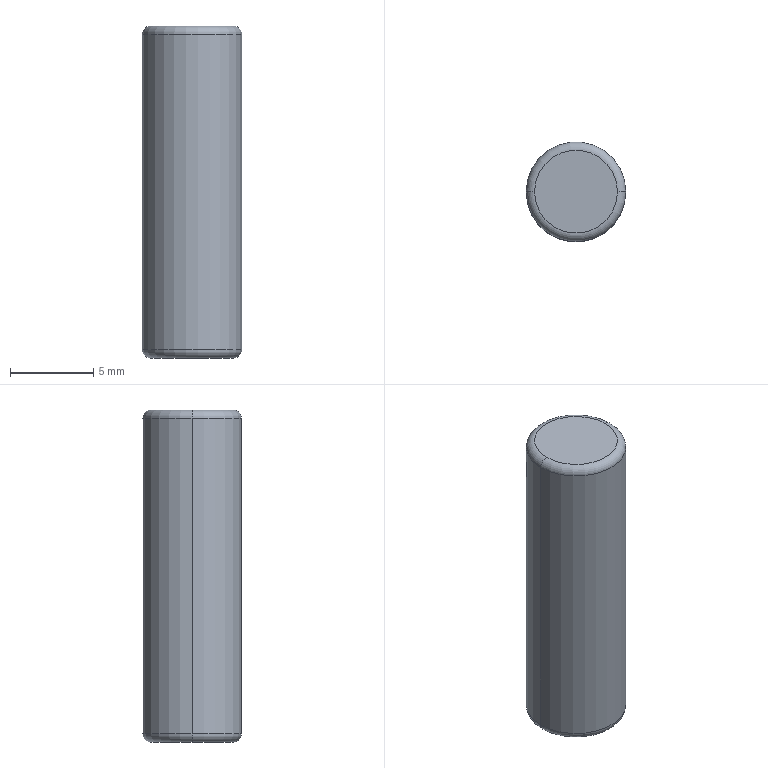Part | STEP file | 1 solid | 8 faces | box 6 x 6 x 20 mm | volume 563.539 mm3 | torus 4 | cylinder 2 | plane 2 | commonest cylinder face diameters 6 x2
STEP:
#1=CARTESIAN_POINT('',(0.,0.,0.));
#2=DIRECTION('',(0.,0.,1.));
#3=DIRECTION('',(1.,0.,0.));
#4=AXIS2_PLACEMENT_3D('',#1,#2,#3);
#5=CARTESIAN_POINT('',(-3.,0.,19.5));
#6=VERTEX_POINT('',#5);
#7=CARTESIAN_POINT('',(3.,0.,19.5));
#8=VERTEX_POINT('',#7);
#9=CARTESIAN_POINT('',(0.,0.,19.5));
#10=DIRECTION('',(0.,0.,-1.));
#11=DIRECTION('',(1.,0.,0.));
#12=AXIS2_PLACEMENT_3D('',#9,#10,#11);
#13=CIRCLE('',#12,3.);
#14=CARTESIAN_POINT('',(0.,0.,19.5));
#15=DIRECTION('',(0.,0.,1.));
#16=DIRECTION('',(1.,0.,0.));
#17=AXIS2_PLACEMENT_3D('',#14,#15,#16);
#18=TOROIDAL_SURFACE('',#17,2.5,0.5);
#19=CARTESIAN_POINT('',(6.283,0.));
#20=DIRECTION('',(-1.,0.));
#21=VECTOR('',#20,1.);
#22=LINE('',#19,#21);
#23=(GEOMETRIC_REPRESENTATION_CONTEXT(2)PARAMETRIC_REPRESENTATION_CONTEXT()REPRESENTATION_CONTEXT('',''));
#24=DEFINITIONAL_REPRESENTATION('',(#22),#23);
#25=PCURVE('',#18,#24);
#26=CARTESIAN_POINT('',(0.,0.,20.));
#27=DIRECTION('',(0.,0.,-1.));
#28=DIRECTION('',(-1.,0.,0.));
#29=AXIS2_PLACEMENT_3D('',#26,#27,#28);
#30=CYLINDRICAL_SURFACE('',#29,3.);
#31=CARTESIAN_POINT('',(-3.142,0.5));
#32=DIRECTION('',(1.,0.));
#33=VECTOR('',#32,1.);
#34=LINE('',#31,#33);
#35=(GEOMETRIC_REPRESENTATION_CONTEXT(2)PARAMETRIC_REPRESENTATION_CONTEXT()REPRESENTATION_CONTEXT('',''));
#36=DEFINITIONAL_REPRESENTATION('',(#34),#35);
#37=PCURVE('',#30,#36);
#38=SURFACE_CURVE('',#13,(#25,#37),.PCURVE_S1.);
#39=EDGE_CURVE('',#6,#8,#38,.T.);
#40=ORIENTED_EDGE('',*,*,#39,.F.);
#41=CARTESIAN_POINT('',(-2.5,0.,20.));
#42=VERTEX_POINT('',#41);
#43=CARTESIAN_POINT('',(-2.5,0.,19.5));
#44=DIRECTION('',(0.,1.,0.));
#45=DIRECTION('',(-1.,0.,0.));
#46=AXIS2_PLACEMENT_3D('',#43,#44,#45);
#47=CIRCLE('',#46,0.5);
#48=CARTESIAN_POINT('',(3.142,0.));
#49=DIRECTION('',(0.,1.));
#50=VECTOR('',#49,1.);
#51=LINE('',#48,#50);
#52=(GEOMETRIC_REPRESENTATION_CONTEXT(2)PARAMETRIC_REPRESENTATION_CONTEXT()REPRESENTATION_CONTEXT('',''));
#53=DEFINITIONAL_REPRESENTATION('',(#51),#52);
#54=PCURVE('',#18,#53);
#55=CARTESIAN_POINT('',(0.,0.,19.5));
#56=DIRECTION('',(0.,0.,1.));
#57=DIRECTION('',(1.,0.,0.));
#58=AXIS2_PLACEMENT_3D('',#55,#56,#57);
#59=TOROIDAL_SURFACE('',#58,2.5,0.5);
#60=CARTESIAN_POINT('',(3.142,0.));
#61=DIRECTION('',(0.,1.));
#62=VECTOR('',#61,1.);
#63=LINE('',#60,#62);
#64=(GEOMETRIC_REPRESENTATION_CONTEXT(2)PARAMETRIC_REPRESENTATION_CONTEXT()REPRESENTATION_CONTEXT('',''));
#65=DEFINITIONAL_REPRESENTATION('',(#63),#64);
#66=PCURVE('',#59,#65);
#67=SURFACE_CURVE('',#47,(#54,#66),.PCURVE_S1.);
#68=EDGE_CURVE('',#6,#42,#67,.T.);
#69=ORIENTED_EDGE('',*,*,#68,.T.);
#70=CARTESIAN_POINT('',(2.5,0.,20.));
#71=VERTEX_POINT('',#70);
#72=CARTESIAN_POINT('',(0.,0.,20.));
#73=DIRECTION('',(0.,0.,1.));
#74=DIRECTION('',(1.,0.,0.));
#75=AXIS2_PLACEMENT_3D('',#72,#73,#74);
#76=CIRCLE('',#75,2.5);
#77=CARTESIAN_POINT('',(0.,1.571));
#78=DIRECTION('',(1.,0.));
#79=VECTOR('',#78,1.);
#80=LINE('',#77,#79);
#81=(GEOMETRIC_REPRESENTATION_CONTEXT(2)PARAMETRIC_REPRESENTATION_CONTEXT()REPRESENTATION_CONTEXT('',''));
#82=DEFINITIONAL_REPRESENTATION('',(#80),#81);
#83=PCURVE('',#18,#82);
#84=CARTESIAN_POINT('',(0.,0.,20.));
#85=DIRECTION('',(0.,0.,1.));
#86=DIRECTION('',(1.,0.,0.));
#87=AXIS2_PLACEMENT_3D('',#84,#85,#86);
#88=PLANE('',#87);
#89=CARTESIAN_POINT('',(0.,0.));
#90=DIRECTION('',(1.,0.));
#91=AXIS2_PLACEMENT_2D('',#89,#90);
#92=CIRCLE('',#91,2.5);
#93=(GEOMETRIC_REPRESENTATION_CONTEXT(2)PARAMETRIC_REPRESENTATION_CONTEXT()REPRESENTATION_CONTEXT('',''));
#94=DEFINITIONAL_REPRESENTATION('',(#92),#93);
#95=PCURVE('',#88,#94);
#96=SURFACE_CURVE('',#76,(#83,#95),.PCURVE_S1.);
#97=EDGE_CURVE('',#71,#42,#96,.T.);
#98=ORIENTED_EDGE('',*,*,#97,.F.);
#99=CARTESIAN_POINT('',(2.5,0.,19.5));
#100=DIRECTION('',(0.,-1.,0.));
#101=DIRECTION('',(0.,0.,-1.));
#102=AXIS2_PLACEMENT_3D('',#99,#100,#101);
#103=CIRCLE('',#102,0.5);
#104=CARTESIAN_POINT('',(0.,-1.571));
#105=DIRECTION('',(0.,1.));
#106=VECTOR('',#105,1.);
#107=LINE('',#104,#106);
#108=(GEOMETRIC_REPRESENTATION_CONTEXT(2)PARAMETRIC_REPRESENTATION_CONTEXT()REPRESENTATION_CONTEXT('',''));
#109=DEFINITIONAL_REPRESENTATION('',(#107),#108);
#110=PCURVE('',#18,#109);
#111=CARTESIAN_POINT('',(6.283,-1.571));
#112=DIRECTION('',(0.,1.));
#113=VECTOR('',#112,1.);
#114=LINE('',#111,#113);
#115=(GEOMETRIC_REPRESENTATION_CONTEXT(2)PARAMETRIC_REPRESENTATION_CONTEXT()REPRESENTATION_CONTEXT('',''));
#116=DEFINITIONAL_REPRESENTATION('',(#114),#115);
#117=PCURVE('',#59,#116);
#118=SURFACE_CURVE('',#103,(#110,#117),.PCURVE_S1.);
#119=EDGE_CURVE('',#8,#71,#118,.T.);
#120=ORIENTED_EDGE('',*,*,#119,.F.);
#121=EDGE_LOOP('',(#40,#69,#98,#120));
#122=FACE_BOUND('',#121,.T.);
#123=ADVANCED_FACE('',(#122),#18,.T.);
#124=CARTESIAN_POINT('',(-2.5,0.,0.));
#125=VERTEX_POINT('',#124);
#126=CARTESIAN_POINT('',(2.5,0.,0.));
#127=VERTEX_POINT('',#126);
#128=CARTESIAN_POINT('',(0.,0.,0.));
#129=DIRECTION('',(0.,0.,-1.));
#130=DIRECTION('',(1.,0.,0.));
#131=AXIS2_PLACEMENT_3D('',#128,#129,#130);
#132=CIRCLE('',#131,2.5);
#133=CARTESIAN_POINT('',(0.,0.,0.5));
#134=DIRECTION('',(0.,0.,1.));
#135=DIRECTION('',(1.,0.,0.));
#136=AXIS2_PLACEMENT_3D('',#133,#134,#135);
#137=TOROIDAL_SURFACE('',#136,2.5,0.5);
#138=CARTESIAN_POINT('',(6.283,4.712));
#139=DIRECTION('',(-1.,0.));
#140=VECTOR('',#139,1.);
#141=LINE('',#138,#140);
#142=(GEOMETRIC_REPRESENTATION_CONTEXT(2)PARAMETRIC_REPRESENTATION_CONTEXT()REPRESENTATION_CONTEXT('',''));
#143=DEFINITIONAL_REPRESENTATION('',(#141),#142);
#144=PCURVE('',#137,#143);
#145=CARTESIAN_POINT('',(0.,0.,0.));
#146=DIRECTION('',(0.,0.,1.));
#147=DIRECTION('',(1.,0.,0.));
#148=AXIS2_PLACEMENT_3D('',#145,#146,#147);
#149=PLANE('',#148);
#150=CARTESIAN_POINT('',(2.5,0.));
#151=CARTESIAN_POINT('',(2.5,-4.33));
#152=CARTESIAN_POINT('',(-1.25,-2.165));
#153=CARTESIAN_POINT('',(-5.,0.));
#154=CARTESIAN_POINT('',(-1.25,2.165));
#155=CARTESIAN_POINT('',(2.5,4.33));
#156=CARTESIAN_POINT('',(2.5,0.));
#157=(BOUNDED_CURVE()B_SPLINE_CURVE(2,(#150,#151,#152,#153,#154,#155,#156),.UNSPECIFIED.,.T.,.F.)B_SPLINE_CURVE_WITH_KNOTS((1,2,2,2,2,1),(-2.094,0.,2.094,4.189,6.283,8.378),.UNSPECIFIED.)CURVE()GEOMETRIC_REPRESENTATION_ITEM()RATIONAL_B_SPLINE_CURVE((1.,0.5,1.,0.5,1.,0.5,1.))REPRESENTATION_ITEM(''));
#158=(GEOMETRIC_REPRESENTATION_CONTEXT(2)PARAMETRIC_REPRESENTATION_CONTEXT()REPRESENTATION_CONTEXT('',''));
#159=DEFINITIONAL_REPRESENTATION('',(#157),#158);
#160=PCURVE('',#149,#159);
#161=SURFACE_CURVE('',#132,(#144,#160),.PCURVE_S1.);
#162=EDGE_CURVE('',#125,#127,#161,.T.);
#163=ORIENTED_EDGE('',*,*,#162,.F.);
#164=CARTESIAN_POINT('',(-3.,0.,0.5));
#165=VERTEX_POINT('',#164);
#166=CARTESIAN_POINT('',(-2.5,0.,0.5));
#167=DIRECTION('',(0.,1.,0.));
#168=DIRECTION('',(-1.,0.,0.));
#169=AXIS2_PLACEMENT_3D('',#166,#167,#168);
#170=CIRCLE('',#169,0.5);
#171=CARTESIAN_POINT('',(3.142,0.));
#172=DIRECTION('',(0.,1.));
#173=VECTOR('',#172,1.);
#174=LINE('',#171,#173);
#175=(GEOMETRIC_REPRESENTATION_CONTEXT(2)PARAMETRIC_REPRESENTATION_CONTEXT()REPRESENTATION_CONTEXT('',''));
#176=DEFINITIONAL_REPRESENTATION('',(#174),#175);
#177=PCURVE('',#137,#176);
#178=CARTESIAN_POINT('',(0.,0.,0.5));
#179=DIRECTION('',(0.,0.,1.));
#180=DIRECTION('',(1.,0.,0.));
#181=AXIS2_PLACEMENT_3D('',#178,#179,#180);
#182=TOROIDAL_SURFACE('',#181,2.5,0.5);
#183=CARTESIAN_POINT('',(3.142,0.));
#184=DIRECTION('',(0.,1.));
#185=VECTOR('',#184,1.);
#186=LINE('',#183,#185);
#187=(GEOMETRIC_REPRESENTATION_CONTEXT(2)PARAMETRIC_REPRESENTATION_CONTEXT()REPRESENTATION_CONTEXT('',''));
#188=DEFINITIONAL_REPRESENTATION('',(#186),#187);
#189=PCURVE('',#182,#188);
#190=SURFACE_CURVE('',#170,(#177,#189),.PCURVE_S1.);
#191=EDGE_CURVE('',#125,#165,#190,.T.);
#192=ORIENTED_EDGE('',*,*,#191,.T.);
#193=CARTESIAN_POINT('',(3.,0.,0.5));
#194=VERTEX_POINT('',#193);
#195=CARTESIAN_POINT('',(0.,0.,0.5));
#196=DIRECTION('',(0.,0.,1.));
#197=DIRECTION('',(1.,0.,0.));
#198=AXIS2_PLACEMENT_3D('',#195,#196,#197);
#199=CIRCLE('',#198,3.);
#200=CARTESIAN_POINT('',(0.,6.283));
#201=DIRECTION('',(1.,0.));
#202=VECTOR('',#201,1.);
#203=LINE('',#200,#202);
#204=(GEOMETRIC_REPRESENTATION_CONTEXT(2)PARAMETRIC_REPRESENTATION_CONTEXT()REPRESENTATION_CONTEXT('',''));
#205=DEFINITIONAL_REPRESENTATION('',(#203),#204);
#206=PCURVE('',#137,#205);
#207=CARTESIAN_POINT('',(3.142,19.5));
#208=DIRECTION('',(-1.,0.));
#209=VECTOR('',#208,1.);
#210=LINE('',#207,#209);
#211=(GEOMETRIC_REPRESENTATION_CONTEXT(2)PARAMETRIC_REPRESENTATION_CONTEXT()REPRESENTATION_CONTEXT('',''));
#212=DEFINITIONAL_REPRESENTATION('',(#210),#211);
#213=PCURVE('',#30,#212);
#214=SURFACE_CURVE('',#199,(#206,#213),.PCURVE_S1.);
#215=EDGE_CURVE('',#194,#165,#214,.T.);
#216=ORIENTED_EDGE('',*,*,#215,.F.);
#217=CARTESIAN_POINT('',(2.5,0.,0.5));
#218=DIRECTION('',(0.,-1.,0.));
#219=DIRECTION('',(0.,0.,-1.));
#220=AXIS2_PLACEMENT_3D('',#217,#218,#219);
#221=CIRCLE('',#220,0.5);
#222=CARTESIAN_POINT('',(0.,4.712));
#223=DIRECTION('',(0.,1.));
#224=VECTOR('',#223,1.);
#225=LINE('',#222,#224);
#226=(GEOMETRIC_REPRESENTATION_CONTEXT(2)PARAMETRIC_REPRESENTATION_CONTEXT()REPRESENTATION_CONTEXT('',''));
#227=DEFINITIONAL_REPRESENTATION('',(#225),#226);
#228=PCURVE('',#137,#227);
#229=CARTESIAN_POINT('',(6.283,4.712));
#230=DIRECTION('',(0.,1.));
#231=VECTOR('',#230,1.);
#232=LINE('',#229,#231);
#233=(GEOMETRIC_REPRESENTATION_CONTEXT(2)PARAMETRIC_REPRESENTATION_CONTEXT()REPRESENTATION_CONTEXT('',''));
#234=DEFINITIONAL_REPRESENTATION('',(#232),#233);
#235=PCURVE('',#182,#234);
#236=SURFACE_CURVE('',#221,(#228,#235),.PCURVE_S1.);
#237=EDGE_CURVE('',#127,#194,#236,.T.);
#238=ORIENTED_EDGE('',*,*,#237,.F.);
#239=EDGE_LOOP('',(#163,#192,#216,#238));
#240=FACE_BOUND('',#239,.T.);
#241=ADVANCED_FACE('',(#240),#137,.T.);
#242=ORIENTED_EDGE('',*,*,#39,.T.);
#243=CARTESIAN_POINT('',(3.,0.,20.));
#244=DIRECTION('',(0.,0.,-1.));
#245=VECTOR('',#244,1.);
#246=LINE('',#243,#245);
#247=CARTESIAN_POINT('',(3.142,0.));
#248=DIRECTION('',(0.,1.));
#249=VECTOR('',#248,1.);
#250=LINE('',#247,#249);
#251=(GEOMETRIC_REPRESENTATION_CONTEXT(2)PARAMETRIC_REPRESENTATION_CONTEXT()REPRESENTATION_CONTEXT('',''));
#252=DEFINITIONAL_REPRESENTATION('',(#250),#251);
#253=PCURVE('',#30,#252);
#254=CARTESIAN_POINT('',(0.,0.,20.));
#255=DIRECTION('',(0.,0.,-1.));
#256=DIRECTION('',(-1.,0.,0.));
#257=AXIS2_PLACEMENT_3D('',#254,#255,#256);
#258=CYLINDRICAL_SURFACE('',#257,3.);
#259=CARTESIAN_POINT('',(3.142,0.));
#260=DIRECTION('',(0.,1.));
#261=VECTOR('',#260,1.);
#262=LINE('',#259,#261);
#263=(GEOMETRIC_REPRESENTATION_CONTEXT(2)PARAMETRIC_REPRESENTATION_CONTEXT()REPRESENTATION_CONTEXT('',''));
#264=DEFINITIONAL_REPRESENTATION('',(#262),#263);
#265=PCURVE('',#258,#264);
#266=SURFACE_CURVE('',#246,(#253,#265),.PCURVE_S1.);
#267=EDGE_CURVE('',#8,#194,#266,.T.);
#268=ORIENTED_EDGE('',*,*,#267,.T.);
#269=ORIENTED_EDGE('',*,*,#215,.T.);
#270=CARTESIAN_POINT('',(-3.,0.,20.));
#271=DIRECTION('',(0.,0.,-1.));
#272=VECTOR('',#271,1.);
#273=LINE('',#270,#272);
#274=CARTESIAN_POINT('',(0.,0.));
#275=DIRECTION('',(0.,1.));
#276=VECTOR('',#275,1.);
#277=LINE('',#274,#276);
#278=(GEOMETRIC_REPRESENTATION_CONTEXT(2)PARAMETRIC_REPRESENTATION_CONTEXT()REPRESENTATION_CONTEXT('',''));
#279=DEFINITIONAL_REPRESENTATION('',(#277),#278);
#280=PCURVE('',#30,#279);
#281=CARTESIAN_POINT('',(6.283,0.));
#282=DIRECTION('',(0.,1.));
#283=VECTOR('',#282,1.);
#284=LINE('',#281,#283);
#285=(GEOMETRIC_REPRESENTATION_CONTEXT(2)PARAMETRIC_REPRESENTATION_CONTEXT()REPRESENTATION_CONTEXT('',''));
#286=DEFINITIONAL_REPRESENTATION('',(#284),#285);
#287=PCURVE('',#258,#286);
#288=SURFACE_CURVE('',#273,(#280,#287),.PCURVE_S1.);
#289=EDGE_CURVE('',#6,#165,#288,.T.);
#290=ORIENTED_EDGE('',*,*,#289,.F.);
#291=EDGE_LOOP('',(#242,#268,#269,#290));
#292=FACE_BOUND('',#291,.T.);
#293=ADVANCED_FACE('',(#292),#30,.T.);
#294=ORIENTED_EDGE('',*,*,#267,.F.);
#295=CARTESIAN_POINT('',(0.,0.,19.5));
#296=DIRECTION('',(0.,0.,-1.));
#297=DIRECTION('',(1.,0.,0.));
#298=AXIS2_PLACEMENT_3D('',#295,#296,#297);
#299=CIRCLE('',#298,3.);
#300=CARTESIAN_POINT('',(3.142,0.5));
#301=DIRECTION('',(1.,0.));
#302=VECTOR('',#301,1.);
#303=LINE('',#300,#302);
#304=(GEOMETRIC_REPRESENTATION_CONTEXT(2)PARAMETRIC_REPRESENTATION_CONTEXT()REPRESENTATION_CONTEXT('',''));
#305=DEFINITIONAL_REPRESENTATION('',(#303),#304);
#306=PCURVE('',#258,#305);
#307=CARTESIAN_POINT('',(6.283,0.));
#308=DIRECTION('',(-1.,0.));
#309=VECTOR('',#308,1.);
#310=LINE('',#307,#309);
#311=(GEOMETRIC_REPRESENTATION_CONTEXT(2)PARAMETRIC_REPRESENTATION_CONTEXT()REPRESENTATION_CONTEXT('',''));
#312=DEFINITIONAL_REPRESENTATION('',(#310),#311);
#313=PCURVE('',#59,#312);
#314=SURFACE_CURVE('',#299,(#306,#313),.PCURVE_S1.);
#315=EDGE_CURVE('',#8,#6,#314,.T.);
#316=ORIENTED_EDGE('',*,*,#315,.T.);
#317=ORIENTED_EDGE('',*,*,#289,.T.);
#318=CARTESIAN_POINT('',(0.,0.,0.5));
#319=DIRECTION('',(0.,0.,1.));
#320=DIRECTION('',(1.,0.,0.));
#321=AXIS2_PLACEMENT_3D('',#318,#319,#320);
#322=CIRCLE('',#321,3.);
#323=CARTESIAN_POINT('',(9.425,19.5));
#324=DIRECTION('',(-1.,0.));
#325=VECTOR('',#324,1.);
#326=LINE('',#323,#325);
#327=(GEOMETRIC_REPRESENTATION_CONTEXT(2)PARAMETRIC_REPRESENTATION_CONTEXT()REPRESENTATION_CONTEXT('',''));
#328=DEFINITIONAL_REPRESENTATION('',(#326),#327);
#329=PCURVE('',#258,#328);
#330=CARTESIAN_POINT('',(0.,6.283));
#331=DIRECTION('',(1.,0.));
#332=VECTOR('',#331,1.);
#333=LINE('',#330,#332);
#334=(GEOMETRIC_REPRESENTATION_CONTEXT(2)PARAMETRIC_REPRESENTATION_CONTEXT()REPRESENTATION_CONTEXT('',''));
#335=DEFINITIONAL_REPRESENTATION('',(#333),#334);
#336=PCURVE('',#182,#335);
#337=SURFACE_CURVE('',#322,(#329,#336),.PCURVE_S1.);
#338=EDGE_CURVE('',#165,#194,#337,.T.);
#339=ORIENTED_EDGE('',*,*,#338,.T.);
#340=EDGE_LOOP('',(#294,#316,#317,#339));
#341=FACE_BOUND('',#340,.T.);
#342=ADVANCED_FACE('',(#341),#258,.T.);
#343=ORIENTED_EDGE('',*,*,#97,.T.);
#344=CARTESIAN_POINT('',(0.,0.,20.));
#345=DIRECTION('',(0.,0.,1.));
#346=DIRECTION('',(1.,0.,0.));
#347=AXIS2_PLACEMENT_3D('',#344,#345,#346);
#348=CIRCLE('',#347,2.5);
#349=CARTESIAN_POINT('',(0.,0.));
#350=DIRECTION('',(1.,0.));
#351=AXIS2_PLACEMENT_2D('',#349,#350);
#352=CIRCLE('',#351,2.5);
#353=(GEOMETRIC_REPRESENTATION_CONTEXT(2)PARAMETRIC_REPRESENTATION_CONTEXT()REPRESENTATION_CONTEXT('',''));
#354=DEFINITIONAL_REPRESENTATION('',(#352),#353);
#355=PCURVE('',#88,#354);
#356=CARTESIAN_POINT('',(0.,1.571));
#357=DIRECTION('',(1.,0.));
#358=VECTOR('',#357,1.);
#359=LINE('',#356,#358);
#360=(GEOMETRIC_REPRESENTATION_CONTEXT(2)PARAMETRIC_REPRESENTATION_CONTEXT()REPRESENTATION_CONTEXT('',''));
#361=DEFINITIONAL_REPRESENTATION('',(#359),#360);
#362=PCURVE('',#59,#361);
#363=SURFACE_CURVE('',#348,(#355,#362),.PCURVE_S1.);
#364=EDGE_CURVE('',#42,#71,#363,.T.);
#365=ORIENTED_EDGE('',*,*,#364,.T.);
#366=EDGE_LOOP('',(#343,#365));
#367=FACE_BOUND('',#366,.T.);
#368=ADVANCED_FACE('',(#367),#88,.T.);
#369=CARTESIAN_POINT('',(0.,0.,0.));
#370=DIRECTION('',(0.,0.,-1.));
#371=DIRECTION('',(1.,0.,0.));
#372=AXIS2_PLACEMENT_3D('',#369,#370,#371);
#373=CIRCLE('',#372,2.5);
#374=CARTESIAN_POINT('',(2.5,0.));
#375=CARTESIAN_POINT('',(2.5,-4.33));
#376=CARTESIAN_POINT('',(-1.25,-2.165));
#377=CARTESIAN_POINT('',(-5.,0.));
#378=CARTESIAN_POINT('',(-1.25,2.165));
#379=CARTESIAN_POINT('',(2.5,4.33));
#380=CARTESIAN_POINT('',(2.5,0.));
#381=(BOUNDED_CURVE()B_SPLINE_CURVE(2,(#374,#375,#376,#377,#378,#379,#380),.UNSPECIFIED.,.T.,.F.)B_SPLINE_CURVE_WITH_KNOTS((1,2,2,2,2,1),(-2.094,0.,2.094,4.189,6.283,8.378),.UNSPECIFIED.)CURVE()GEOMETRIC_REPRESENTATION_ITEM()RATIONAL_B_SPLINE_CURVE((1.,0.5,1.,0.5,1.,0.5,1.))REPRESENTATION_ITEM(''));
#382=(GEOMETRIC_REPRESENTATION_CONTEXT(2)PARAMETRIC_REPRESENTATION_CONTEXT()REPRESENTATION_CONTEXT('',''));
#383=DEFINITIONAL_REPRESENTATION('',(#381),#382);
#384=PCURVE('',#149,#383);
#385=CARTESIAN_POINT('',(6.283,4.712));
#386=DIRECTION('',(-1.,0.));
#387=VECTOR('',#386,1.);
#388=LINE('',#385,#387);
#389=(GEOMETRIC_REPRESENTATION_CONTEXT(2)PARAMETRIC_REPRESENTATION_CONTEXT()REPRESENTATION_CONTEXT('',''));
#390=DEFINITIONAL_REPRESENTATION('',(#388),#389);
#391=PCURVE('',#182,#390);
#392=SURFACE_CURVE('',#373,(#384,#391),.PCURVE_S1.);
#393=EDGE_CURVE('',#127,#125,#392,.T.);
#394=ORIENTED_EDGE('',*,*,#393,.T.);
#395=ORIENTED_EDGE('',*,*,#162,.T.);
#396=EDGE_LOOP('',(#394,#395));
#397=FACE_BOUND('',#396,.T.);
#398=ADVANCED_FACE('',(#397),#149,.F.);
#399=ORIENTED_EDGE('',*,*,#191,.F.);
#400=ORIENTED_EDGE('',*,*,#393,.F.);
#401=ORIENTED_EDGE('',*,*,#237,.T.);
#402=ORIENTED_EDGE('',*,*,#338,.F.);
#403=EDGE_LOOP('',(#399,#400,#401,#402));
#404=FACE_BOUND('',#403,.T.);
#405=ADVANCED_FACE('',(#404),#182,.T.);
#406=ORIENTED_EDGE('',*,*,#68,.F.);
#407=ORIENTED_EDGE('',*,*,#315,.F.);
#408=ORIENTED_EDGE('',*,*,#119,.T.);
#409=ORIENTED_EDGE('',*,*,#364,.F.);
#410=EDGE_LOOP('',(#406,#407,#408,#409));
#411=FACE_BOUND('',#410,.T.);
#412=ADVANCED_FACE('',(#411),#59,.T.);
#413=CLOSED_SHELL('',(#123,#241,#293,#342,#368,#398,#405,#412));
#414=MANIFOLD_SOLID_BREP('',#413);
#415=(LENGTH_UNIT()NAMED_UNIT(*)SI_UNIT(.MILLI.,.METRE.));
#416=UNCERTAINTY_MEASURE_WITH_UNIT(LENGTH_MEASURE(0.0000001),#415,'','');
#417=(NAMED_UNIT(*)PLANE_ANGLE_UNIT()SI_UNIT($,.RADIAN.));
#418=(NAMED_UNIT(*)SI_UNIT($,.STERADIAN.)SOLID_ANGLE_UNIT());
#419=(GEOMETRIC_REPRESENTATION_CONTEXT(3)GLOBAL_UNCERTAINTY_ASSIGNED_CONTEXT((#416))GLOBAL_UNIT_ASSIGNED_CONTEXT((#415,#417,#418))REPRESENTATION_CONTEXT('',''));
#420=ADVANCED_BREP_SHAPE_REPRESENTATION('',(#4,#414),#419);